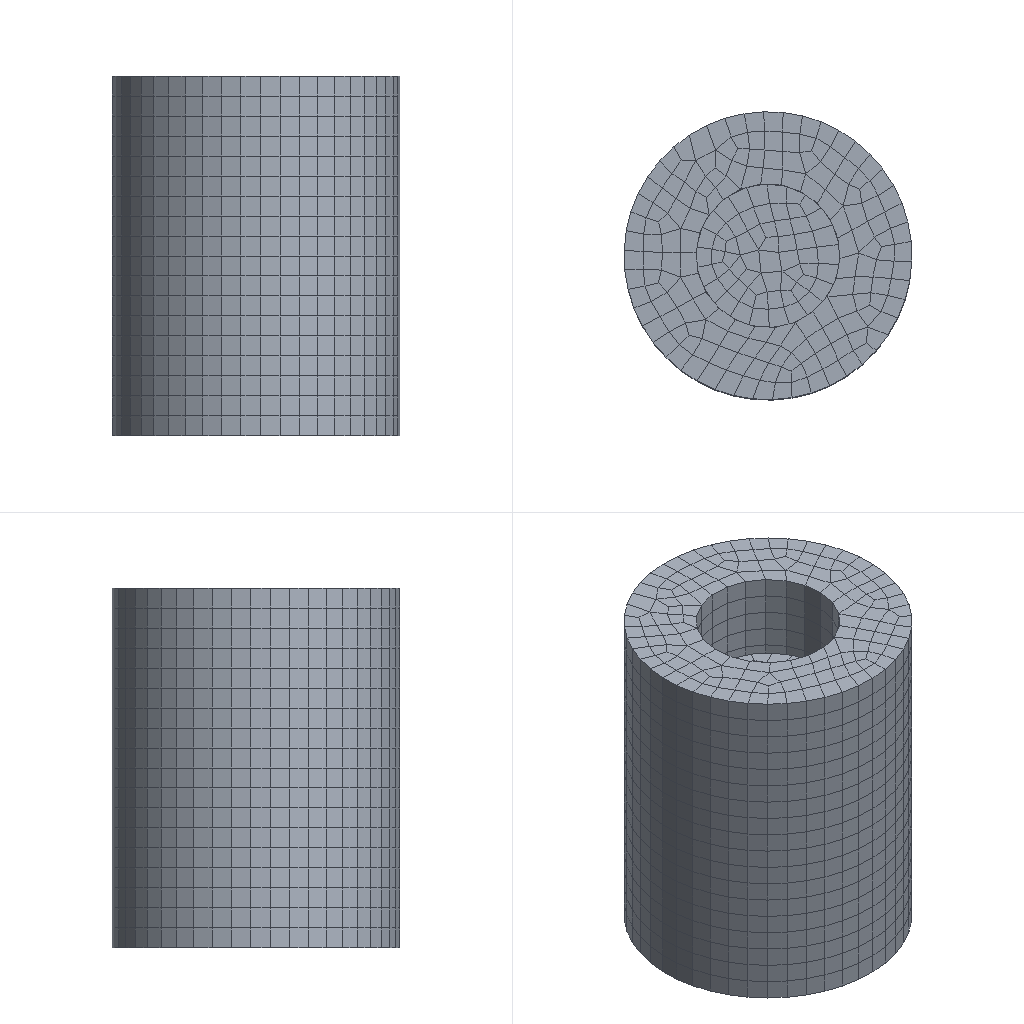Simulation study | abaqus
Set-up summary:
category,name,step,type,value,unit,region
solver,abaqus
solver,version,,,Abaqus/Standard 2020
units,not stated in the deck,,not stated
analysis,deck,,transient,transient
load_step,Step-1,Step-1,transient
load_step,requested,,,1
mesh,nodes,,,4273
mesh,elements,,,3294
element_type,C3D8R,,solid,3294
load,load commands in deck,,count,2
bc,support commands in deck,,count,6
material,MATERIAL-1,,in results
check,setup vs results,,match,"per instance, exact: element labels, types and connectivity; labels of the nodes the elements use; coordinates of those nodes at SINGLE_PRECISION in 2 of 2 instance(s)"
Abaqus input file, long lists of numbers shortened:
*Heading
** Job name: Job-2 Model name: Model-1-Copy
** Generated by: Abaqus/CAE 2020
*Preprint, echo=NO, model=NO, history=NO, contact=NO
**
** PARTS
**
*Part, name=Part-1
*Node
      1,   7.666,  -6.421,           0.
      2,   9.165,  -4.001,           0.
** (718 more lines like these left out)
*Element, type=C3D8R
  1,  95,  92,  91,  96,  23,  20,  19,  24
  2,  96,  91,  90,  97,  24,  19,  18,  25
** (538 more lines like these left out)
*Nset, nset=Set-1, generate
   1,  720,    1
*Elset, elset=Set-1, generate
   1,  540,    1
** Section: Section-1
*Solid Section, elset=Set-1, material=Material-1
,
*End Part
**
*Part, name=tong
*Node
      1,   8.194,  -5.732,           0.
      2,   9.477,  -3.192,           0.
** (3551 more lines like these left out)
*Element, type=C3D8R
   1,  301,  233,  191,  259,  114,   46,    4,   72
   2,  356,  308,  257,  337,  169,  121,   70,  150
** (2752 more lines like these left out)
*Nset, nset=Set-1, generate
    1,  3553,     1
*Elset, elset=Set-1, generate
    1,  2754,     1
** Section: Section-1
*Solid Section, elset=Set-1, material=Material-1
,
*End Part
**
**
** ASSEMBLY
**
*Assembly, name=Assembly
**
*Instance, name=Part-1-1, part=Part-1
          0.,           0.,         12.5
*End Instance
**
*Instance, name=tong-1, part=tong
*End Instance
**
*Node
      1,           0.,           0.,          25.
*Nset, nset=Set-1, instance=Part-1-1, generate
   1,  720,    1
*Elset, elset=Set-1, instance=Part-1-1, generate
   1,  540,    1
*Nset, nset=Set-3
 1,
*Nset, nset=m_Set-2
 1,
*Elset, elset=_Surf-3_S4, internal, instance=Part-1-1
   1,   2,  17,  18,  19,  20,  21,  22,  24,  25,  26,  61,  62,  77,  78,  79
  80,  81,  82,  84,  85,  86, 121, 122, 137, 138, 139, 140, 141, 142, 144, 145
** (5 more lines like these left out)
*Elset, elset=_Surf-3_S5, internal, instance=Part-1-1
   3,  15,  23,  27,  33,  63,  75,  83,  87,  93, 123, 135, 143, 147, 153, 183
 195, 203, 207, 213, 243, 255, 263, 267, 273, 303, 315, 323, 327, 333, 363, 375
** (1 more lines like these left out)
*Elset, elset=_Surf-3_S3, internal, instance=Part-1-1
   6,  31,  36,  66,  91,  96, 126, 151, 156, 186, 211, 216, 246, 271, 276, 306
 331, 336, 366, 391, 396, 426, 451, 456, 486, 511, 516
*Elset, elset=_Surf-3_S6, internal, instance=Part-1-1
   7,  11,  16,  67,  71,  76, 127, 131, 136, 187, 191, 196, 247, 251, 256, 307
 311, 316, 367, 371, 376, 427, 431, 436, 487, 491, 496
*Surface, type=ELEMENT, name=Surf-3
_Surf-3_S4, S4
_Surf-3_S5, S5
_Surf-3_S6, S6
_Surf-3_S3, S3
*Elset, elset=_m_Surf-1_S4, internal, instance=tong-1
    1,   25,   66,   70,   79,   85,   86,   99,  154,  178,  219,  223,  232,  238,  239,  252
  307,  331,  372,  376,  385,  391,  392,  405,  460,  484,  525,  529,  538,  544,  545,  558
** (7 more lines like these left out)
*Elset, elset=_m_Surf-1_S6, internal, instance=tong-1
    5,    6,    8,   24,   27,   41,   45,  158,  159,  161,  177,  180,  194,  198,  311,  312
  314,  330,  333,  347,  351,  464,  465,  467,  483,  486,  500,  504,  617,  618,  620,  636
** (6 more lines like these left out)
*Elset, elset=_m_Surf-1_S5, internal, instance=tong-1
   13,   35,  166,  188,  319,  341,  472,  494,  625,  647,  778,  800,  931,  953, 1084, 1106
 1237, 1259, 1390, 1412, 1543, 1565, 1696, 1718, 1849, 1871, 2002, 2024, 2155, 2177, 2308, 2330
** (1 more lines like these left out)
*Elset, elset=_m_Surf-1_S3, internal, instance=tong-1
   71,   81,   91,   95,   96,  224,  234,  244,  248,  249,  377,  387,  397,  401,  402,  530
  540,  550,  554,  555,  683,  693,  703,  707,  708,  836,  846,  856,  860,  861,  989,  999
** (4 more lines like these left out)
*Surface, type=ELEMENT, name=m_Surf-1
_m_Surf-1_S4, S4
_m_Surf-1_S6, S6
_m_Surf-1_S5, S5
_m_Surf-1_S3, S3
*Elset, elset=_s_Surf-1_S4, internal, instance=Part-1-1
   1,   2,  17,  18,  19,  20,  21,  22,  24,  25,  26,  61,  62,  77,  78,  79
  80,  81,  82,  84,  85,  86, 121, 122, 137, 138, 139, 140, 141, 142, 144, 145
** (5 more lines like these left out)
*Elset, elset=_s_Surf-1_S5, internal, instance=Part-1-1
   3,  15,  23,  27,  33,  63,  75,  83,  87,  93, 123, 135, 143, 147, 153, 183
 195, 203, 207, 213, 243, 255, 263, 267, 273, 303, 315, 323, 327, 333, 363, 375
** (1 more lines like these left out)
*Elset, elset=_s_Surf-1_S3, internal, instance=Part-1-1
   6,  31,  36,  66,  91,  96, 126, 151, 156, 186, 211, 216, 246, 271, 276, 306
 331, 336, 366, 391, 396, 426, 451, 456, 486, 511, 516
*Elset, elset=_s_Surf-1_S6, internal, instance=Part-1-1
   7,  11,  16,  67,  71,  76, 127, 131, 136, 187, 191, 196, 247, 251, 256, 307
 311, 316, 367, 371, 376, 427, 431, 436, 487, 491, 496
*Surface, type=ELEMENT, name=s_Surf-1
_s_Surf-1_S4, S4
_s_Surf-1_S5, S5
_s_Surf-1_S6, S6
_s_Surf-1_S3, S3
*Elset, elset=_s_Surf-4_S1, internal, instance=Part-1-1, generate
 481,  540,    1
*Elset, elset=_s_Surf-4_S2, internal, instance=Part-1-1, generate
  1,  60,   1
*Surface, type=ELEMENT, name=s_Surf-4
_s_Surf-4_S1, S1
_s_Surf-4_S2, S2
** Constraint: Constraint-1
*Coupling, constraint name=Constraint-1, ref node=m_Set-2, surface=s_Surf-4
*Kinematic
*End Assembly
*Amplitude, name=Amp-1
             0.,              0.,             10.,              1.
**
** MATERIALS
**
*Material, name=Material-1
*Density
 7.8e-09,
*Elastic
210000., 0.3
**
** INTERACTION PROPERTIES
**
*Surface Interaction, name=IntProp-1
1.,
*Friction, slip tolerance=0.005
 0.1,
*Surface Behavior, pressure-overclosure=HARD
**
** INTERACTIONS
**
** Interaction: Int-1
*Contact Pair, interaction=IntProp-1, type=SURFACE TO SURFACE
s_Surf-1, m_Surf-1
** ----------------------------------------------------------------
**
** STEP: Step-1
**
*Step, name=Step-1, nlgeom=YES, inc=1000
*Dynamic
0.1,10.,0.0001
**
** BOUNDARY CONDITIONS
**
** Name: BC-1 Type: 位移/转角
*Boundary, amplitude=Amp-1
Set-3, 1, 1
Set-3, 2, 2
Set-3, 3, 3
Set-3, 4, 4
Set-3, 5, 5
Set-3, 6, 6, 6.28
**
** LOADS
**
** Name: Load-1   Type: Pressure
*Dsload
Surf-3, P, -0.01
**
** OUTPUT REQUESTS
**
*Restart, write, frequency=0
**
** FIELD OUTPUT: F-Output-1
**
*Output, field, frequency=1
*Node Output
A, AR, AT, CF, RF, U, UR, UT
V, VR, VT
*Element Output, directions=YES
E, LE, MISES, MISESMAX, PE, PEEQ, PEMAG, S
*Contact Output
CDISP, CSTRESS
**
** HISTORY OUTPUT: H-Output-1
**
*Output, history, variable=PRESELECT
*End Step
Results summary:
result,step,,completed,increments=68 time=10.0/10.0
result,analysis,,,transient
result,last_loadstep,,,1
result,primary field,,,U
result,reaction total,,FX,-0.00012,model units
result,reaction total,,FY,0.000217,model units
result,reaction total,,FZ,-0.0,model units